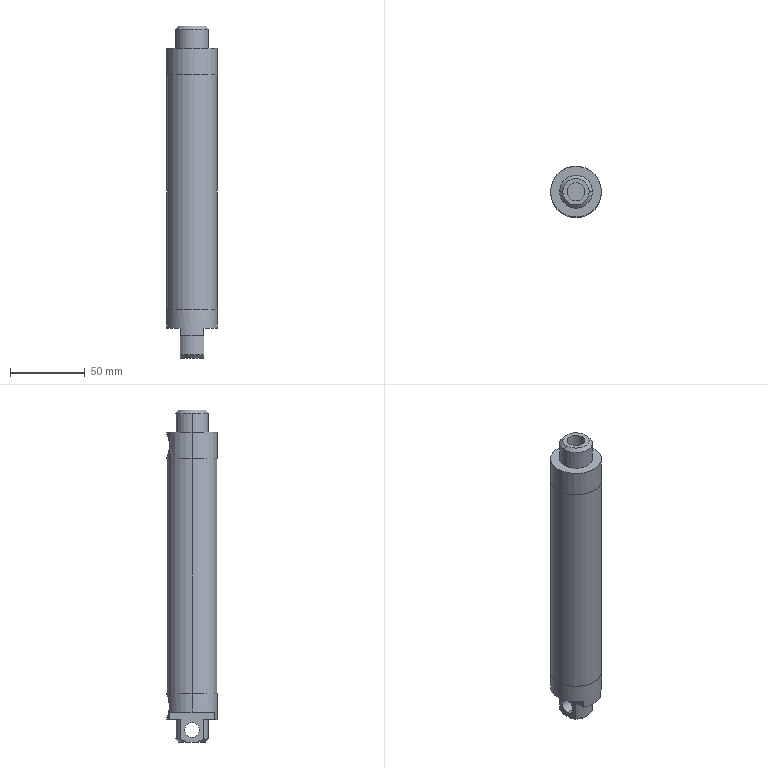Part | STEP file | 1 solid | 49 faces | box 34 x 34 x 222 mm | volume 66628 mm3 | cylinder 24 | plane 17 | cone 8 | commonest cylinder face diameters 7.782 x4 22 x4 34 x4 10 x2 12 x2 15.4 x2